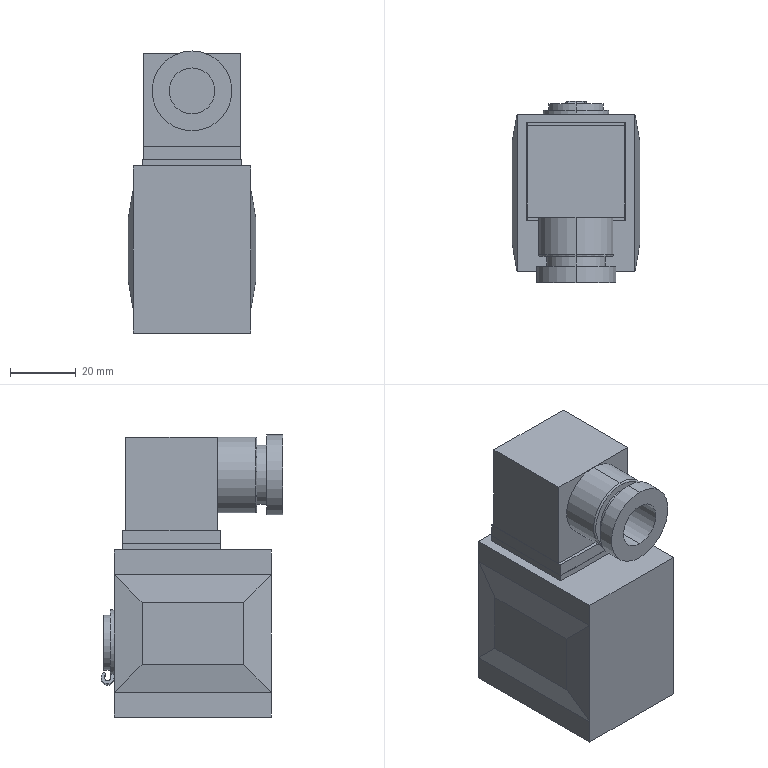Part | STEP file | _2W050-15 - Valve Terminal_3 | 1 solid | 65 faces | box 39 x 55.5 x 86.1 mm | volume 126239 mm3 | plane 42 | cylinder 12 | spline 10 | cone 1 | commonest cylinder face diameters 14 x2 16.8 x2 18 x2 20 x2 23 x2 24.4 x2